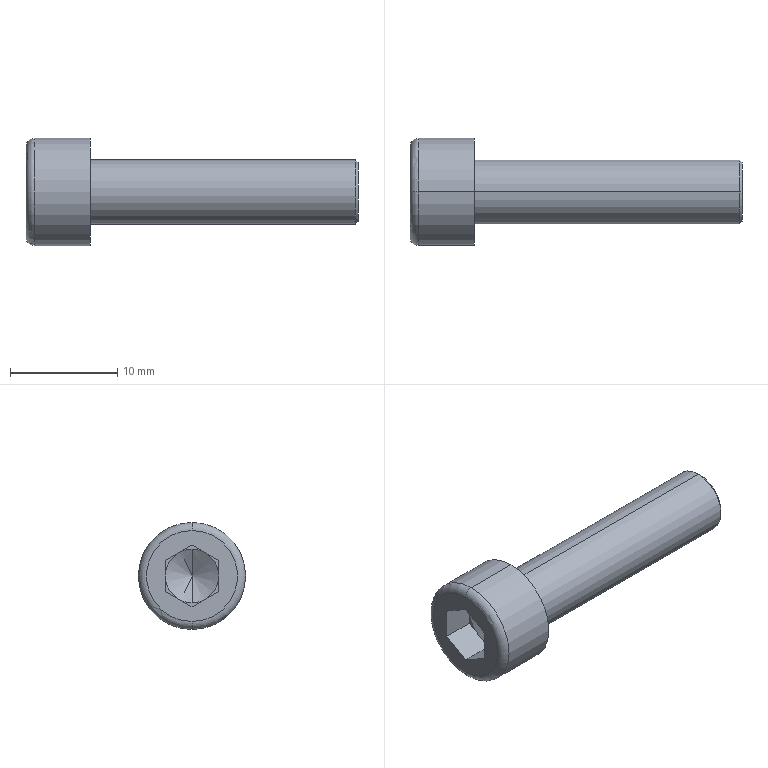Part | SolidWorks | features Fillet 2, RevCut 2, Boss 1, Chamfer 1, Cut 1, Extrusion 1, LPattern 1 | 1 solid | 25 faces | box 31 x 10 x 10 mm | volume 1099 mm3 | plane 15 | cone 4 | cylinder 4 | torus 2 | commonest cylinder face diameters 6 x2 10 x2
STEP:
#1=CARTESIAN_POINT('',(31.,0.,-2.75));
#2=VERTEX_POINT('',#1);
#3=CARTESIAN_POINT('',(31.,0.,2.75));
#4=VERTEX_POINT('',#3);
#5=CARTESIAN_POINT('',(31.,0.,0.));
#6=DIRECTION('',(1.,0.,0.));
#7=DIRECTION('',(0.,0.,-1.));
#8=AXIS2_PLACEMENT_3D('',#5,#6,#7);
#9=CIRCLE('',#8,2.75);
#10=EDGE_CURVE('',#2,#4,#9,.T.);
#11=ORIENTED_EDGE('',*,*,#10,.F.);
#12=CARTESIAN_POINT('',(30.75,0.,-3.));
#13=VERTEX_POINT('',#12);
#14=CARTESIAN_POINT('',(31.,0.,-2.75));
#15=DIRECTION('',(-0.7071,0.,-0.7071));
#16=VECTOR('',#15,1000.);
#17=LINE('',#14,#16);
#18=EDGE_CURVE('',#2,#13,#17,.T.);
#19=ORIENTED_EDGE('',*,*,#18,.T.);
#20=CARTESIAN_POINT('',(30.75,0.,3.));
#21=VERTEX_POINT('',#20);
#22=CARTESIAN_POINT('',(30.75,0.,0.));
#23=DIRECTION('',(-1.,0.,0.));
#24=DIRECTION('',(0.,0.,-1.));
#25=AXIS2_PLACEMENT_3D('',#22,#23,#24);
#26=CIRCLE('',#25,3.);
#27=EDGE_CURVE('',#21,#13,#26,.T.);
#28=ORIENTED_EDGE('',*,*,#27,.F.);
#29=CARTESIAN_POINT('',(31.,0.,2.75));
#30=DIRECTION('',(-0.7071,0.,0.7071));
#31=VECTOR('',#30,1000.);
#32=LINE('',#29,#31);
#33=EDGE_CURVE('',#4,#21,#32,.T.);
#34=ORIENTED_EDGE('',*,*,#33,.F.);
#35=EDGE_LOOP('',(#11,#19,#28,#34));
#36=FACE_OUTER_BOUND('',#35,.T.);
#37=CARTESIAN_POINT('',(31.,0.,0.));
#38=DIRECTION('',(-1.,0.,0.));
#39=DIRECTION('',(0.,0.,1.));
#40=AXIS2_PLACEMENT_3D('',#37,#38,#39);
#41=CONICAL_SURFACE('',#40,2.75,0.7854);
#42=ADVANCED_FACE('',(#36),#41,.T.);
#43=CARTESIAN_POINT('',(0.,0.,4.25));
#44=VERTEX_POINT('',#43);
#45=CARTESIAN_POINT('',(0.,0.,-4.25));
#46=VERTEX_POINT('',#45);
#47=CARTESIAN_POINT('',(0.,0.,0.));
#48=DIRECTION('',(-1.,0.,0.));
#49=DIRECTION('',(0.,0.,-1.));
#50=AXIS2_PLACEMENT_3D('',#47,#48,#49);
#51=CIRCLE('',#50,4.25);
#52=EDGE_CURVE('',#44,#46,#51,.T.);
#53=ORIENTED_EDGE('',*,*,#52,.F.);
#54=CARTESIAN_POINT('',(0.75,0.,5.));
#55=VERTEX_POINT('',#54);
#56=CARTESIAN_POINT('',(0.75,0.,4.25));
#57=DIRECTION('',(0.,1.,0.));
#58=DIRECTION('',(0.,0.,1.));
#59=AXIS2_PLACEMENT_3D('',#56,#57,#58);
#60=CIRCLE('',#59,0.75);
#61=EDGE_CURVE('',#44,#55,#60,.T.);
#62=ORIENTED_EDGE('',*,*,#61,.T.);
#63=CARTESIAN_POINT('',(0.75,0.,-5.));
#64=VERTEX_POINT('',#63);
#65=CARTESIAN_POINT('',(0.75,0.,0.));
#66=DIRECTION('',(1.,0.,0.));
#67=DIRECTION('',(0.,0.,-1.));
#68=AXIS2_PLACEMENT_3D('',#65,#66,#67);
#69=CIRCLE('',#68,5.);
#70=EDGE_CURVE('',#64,#55,#69,.T.);
#71=ORIENTED_EDGE('',*,*,#70,.F.);
#72=CARTESIAN_POINT('',(0.75,0.,-4.25));
#73=DIRECTION('',(0.,-1.,0.));
#74=DIRECTION('',(0.,0.,-1.));
#75=AXIS2_PLACEMENT_3D('',#72,#73,#74);
#76=CIRCLE('',#75,0.75);
#77=EDGE_CURVE('',#46,#64,#76,.T.);
#78=ORIENTED_EDGE('',*,*,#77,.F.);
#79=EDGE_LOOP('',(#53,#62,#71,#78));
#80=FACE_OUTER_BOUND('',#79,.T.);
#81=CARTESIAN_POINT('',(0.75,0.,0.));
#82=DIRECTION('',(1.,0.,0.));
#83=DIRECTION('',(0.,0.,-1.));
#84=AXIS2_PLACEMENT_3D('',#81,#82,#83);
#85=TOROIDAL_SURFACE('',#84,4.25,0.75);
#86=ADVANCED_FACE('',(#80),#85,.T.);
#87=CARTESIAN_POINT('',(4.443,0.,0.));
#88=VERTEX_POINT('',#87);
#89=CARTESIAN_POINT('',(3.,0.,2.5));
#90=VERTEX_POINT('',#89);
#91=CARTESIAN_POINT('',(3.,0.,2.5));
#92=DIRECTION('',(-0.5,0.,0.866));
#93=VECTOR('',#92,1000.);
#94=LINE('',#91,#93);
#95=EDGE_CURVE('',#88,#90,#94,.T.);
#96=ORIENTED_EDGE('',*,*,#95,.F.);
#97=CARTESIAN_POINT('',(3.,0.,-2.5));
#98=VERTEX_POINT('',#97);
#99=CARTESIAN_POINT('',(3.,0.,-2.5));
#100=DIRECTION('',(-0.5,0.,-0.866));
#101=VECTOR('',#100,1000.);
#102=LINE('',#99,#101);
#103=EDGE_CURVE('',#88,#98,#102,.T.);
#104=ORIENTED_EDGE('',*,*,#103,.T.);
#105=CARTESIAN_POINT('',(3.,-1.25,-2.165));
#106=VERTEX_POINT('',#105);
#107=CARTESIAN_POINT('',(3.,0.,0.));
#108=DIRECTION('',(1.,0.,0.));
#109=DIRECTION('',(0.,0.,1.));
#110=AXIS2_PLACEMENT_3D('',#107,#108,#109);
#111=CIRCLE('',#110,2.5);
#112=EDGE_CURVE('',#106,#98,#111,.T.);
#113=ORIENTED_EDGE('',*,*,#112,.F.);
#114=CARTESIAN_POINT('',(3.,-2.5,0.));
#115=VERTEX_POINT('',#114);
#116=CARTESIAN_POINT('',(3.,0.,0.));
#117=DIRECTION('',(1.,0.,0.));
#118=DIRECTION('',(0.,0.,1.));
#119=AXIS2_PLACEMENT_3D('',#116,#117,#118);
#120=CIRCLE('',#119,2.5);
#121=EDGE_CURVE('',#115,#106,#120,.T.);
#122=ORIENTED_EDGE('',*,*,#121,.F.);
#123=CARTESIAN_POINT('',(3.,-1.25,2.165));
#124=VERTEX_POINT('',#123);
#125=CARTESIAN_POINT('',(3.,0.,0.));
#126=DIRECTION('',(1.,0.,0.));
#127=DIRECTION('',(0.,0.,1.));
#128=AXIS2_PLACEMENT_3D('',#125,#126,#127);
#129=CIRCLE('',#128,2.5);
#130=EDGE_CURVE('',#124,#115,#129,.T.);
#131=ORIENTED_EDGE('',*,*,#130,.F.);
#132=CARTESIAN_POINT('',(3.,0.,0.));
#133=DIRECTION('',(1.,0.,0.));
#134=DIRECTION('',(0.,0.,1.));
#135=AXIS2_PLACEMENT_3D('',#132,#133,#134);
#136=CIRCLE('',#135,2.5);
#137=EDGE_CURVE('',#90,#124,#136,.T.);
#138=ORIENTED_EDGE('',*,*,#137,.F.);
#139=EDGE_LOOP('',(#96,#104,#113,#122,#131,#138));
#140=FACE_OUTER_BOUND('',#139,.T.);
#141=CARTESIAN_POINT('',(3.,0.,0.));
#142=DIRECTION('',(-1.,0.,0.));
#143=DIRECTION('',(0.,0.,1.));
#144=AXIS2_PLACEMENT_3D('',#141,#142,#143);
#145=CONICAL_SURFACE('',#144,2.5,1.047);
#146=ADVANCED_FACE('',(#140),#145,.F.);
#147=ORIENTED_EDGE('',*,*,#27,.T.);
#148=CARTESIAN_POINT('',(6.,0.,-3.));
#149=VERTEX_POINT('',#148);
#150=CARTESIAN_POINT('',(31.,0.,-3.));
#151=DIRECTION('',(-1.,0.,0.));
#152=VECTOR('',#151,1000.);
#153=LINE('',#150,#152);
#154=EDGE_CURVE('',#13,#149,#153,.T.);
#155=ORIENTED_EDGE('',*,*,#154,.T.);
#156=CARTESIAN_POINT('',(6.,0.,3.));
#157=VERTEX_POINT('',#156);
#158=CARTESIAN_POINT('',(6.,0.,0.));
#159=DIRECTION('',(1.,0.,0.));
#160=DIRECTION('',(0.,0.,-1.));
#161=AXIS2_PLACEMENT_3D('',#158,#159,#160);
#162=CIRCLE('',#161,3.);
#163=EDGE_CURVE('',#149,#157,#162,.T.);
#164=ORIENTED_EDGE('',*,*,#163,.T.);
#165=CARTESIAN_POINT('',(31.,0.,3.));
#166=DIRECTION('',(-1.,0.,0.));
#167=VECTOR('',#166,1000.);
#168=LINE('',#165,#167);
#169=EDGE_CURVE('',#21,#157,#168,.T.);
#170=ORIENTED_EDGE('',*,*,#169,.F.);
#171=EDGE_LOOP('',(#147,#155,#164,#170));
#172=FACE_OUTER_BOUND('',#171,.T.);
#173=CARTESIAN_POINT('',(31.,0.,0.));
#174=DIRECTION('',(-1.,0.,0.));
#175=DIRECTION('',(0.,0.,1.));
#176=AXIS2_PLACEMENT_3D('',#173,#174,#175);
#177=CYLINDRICAL_SURFACE('',#176,3.);
#178=ADVANCED_FACE('',(#172),#177,.T.);
#179=CARTESIAN_POINT('',(6.,0.,-5.));
#180=VERTEX_POINT('',#179);
#181=CARTESIAN_POINT('',(6.,0.,5.));
#182=VERTEX_POINT('',#181);
#183=CARTESIAN_POINT('',(6.,0.,0.));
#184=DIRECTION('',(1.,0.,0.));
#185=DIRECTION('',(0.,0.,-1.));
#186=AXIS2_PLACEMENT_3D('',#183,#184,#185);
#187=CIRCLE('',#186,5.);
#188=EDGE_CURVE('',#180,#182,#187,.T.);
#189=ORIENTED_EDGE('',*,*,#188,.F.);
#190=CARTESIAN_POINT('',(6.,0.,-5.));
#191=DIRECTION('',(-1.,0.,0.));
#192=VECTOR('',#191,1000.);
#193=LINE('',#190,#192);
#194=EDGE_CURVE('',#180,#64,#193,.T.);
#195=ORIENTED_EDGE('',*,*,#194,.T.);
#196=ORIENTED_EDGE('',*,*,#70,.T.);
#197=CARTESIAN_POINT('',(6.,0.,5.));
#198=DIRECTION('',(-1.,0.,0.));
#199=VECTOR('',#198,1000.);
#200=LINE('',#197,#199);
#201=EDGE_CURVE('',#182,#55,#200,.T.);
#202=ORIENTED_EDGE('',*,*,#201,.F.);
#203=EDGE_LOOP('',(#189,#195,#196,#202));
#204=FACE_OUTER_BOUND('',#203,.T.);
#205=CARTESIAN_POINT('',(6.,0.,0.));
#206=DIRECTION('',(-1.,0.,0.));
#207=DIRECTION('',(0.,0.,1.));
#208=AXIS2_PLACEMENT_3D('',#205,#206,#207);
#209=CYLINDRICAL_SURFACE('',#208,5.);
#210=ADVANCED_FACE('',(#204),#209,.T.);
#211=CARTESIAN_POINT('',(3.,-2.5,1.443));
#212=VERTEX_POINT('',#211);
#213=CARTESIAN_POINT('',(3.,0.,2.887));
#214=DIRECTION('',(0.,-0.866,-0.5));
#215=VECTOR('',#214,1000.);
#216=LINE('',#213,#215);
#217=EDGE_CURVE('',#124,#212,#216,.T.);
#218=ORIENTED_EDGE('',*,*,#217,.F.);
#219=ORIENTED_EDGE('',*,*,#130,.T.);
#220=CARTESIAN_POINT('',(3.,-2.5,1.443));
#221=DIRECTION('',(0.,0.,-1.));
#222=VECTOR('',#221,1000.);
#223=LINE('',#220,#222);
#224=EDGE_CURVE('',#212,#115,#223,.T.);
#225=ORIENTED_EDGE('',*,*,#224,.F.);
#226=EDGE_LOOP('',(#218,#219,#225));
#227=FACE_OUTER_BOUND('',#226,.T.);
#228=CARTESIAN_POINT('',(3.,-5.,0.));
#229=DIRECTION('',(-1.,0.,0.));
#230=DIRECTION('',(0.,0.,1.));
#231=AXIS2_PLACEMENT_3D('',#228,#229,#230);
#232=PLANE('',#231);
#233=ADVANCED_FACE('',(#227),#232,.T.);
#234=CARTESIAN_POINT('',(3.,-2.5,-1.443));
#235=VERTEX_POINT('',#234);
#236=CARTESIAN_POINT('',(3.,-2.5,1.443));
#237=DIRECTION('',(0.,0.,-1.));
#238=VECTOR('',#237,1000.);
#239=LINE('',#236,#238);
#240=EDGE_CURVE('',#115,#235,#239,.T.);
#241=ORIENTED_EDGE('',*,*,#240,.F.);
#242=ORIENTED_EDGE('',*,*,#121,.T.);
#243=CARTESIAN_POINT('',(3.,-2.5,-1.443));
#244=DIRECTION('',(0.,0.866,-0.5));
#245=VECTOR('',#244,1000.);
#246=LINE('',#243,#245);
#247=EDGE_CURVE('',#235,#106,#246,.T.);
#248=ORIENTED_EDGE('',*,*,#247,.F.);
#249=EDGE_LOOP('',(#241,#242,#248));
#250=FACE_OUTER_BOUND('',#249,.T.);
#251=CARTESIAN_POINT('',(3.,-5.,0.));
#252=DIRECTION('',(-1.,0.,0.));
#253=DIRECTION('',(0.,0.,1.));
#254=AXIS2_PLACEMENT_3D('',#251,#252,#253);
#255=PLANE('',#254);
#256=ADVANCED_FACE('',(#250),#255,.T.);
#257=CARTESIAN_POINT('',(3.,0.,-2.887));
#258=VERTEX_POINT('',#257);
#259=CARTESIAN_POINT('',(3.,-2.5,-1.443));
#260=DIRECTION('',(0.,0.866,-0.5));
#261=VECTOR('',#260,1000.);
#262=LINE('',#259,#261);
#263=EDGE_CURVE('',#106,#258,#262,.T.);
#264=ORIENTED_EDGE('',*,*,#263,.F.);
#265=ORIENTED_EDGE('',*,*,#112,.T.);
#266=CARTESIAN_POINT('',(3.,1.25,-2.165));
#267=VERTEX_POINT('',#266);
#268=CARTESIAN_POINT('',(3.,0.,0.));
#269=DIRECTION('',(1.,0.,0.));
#270=DIRECTION('',(0.,0.,1.));
#271=AXIS2_PLACEMENT_3D('',#268,#269,#270);
#272=CIRCLE('',#271,2.5);
#273=EDGE_CURVE('',#98,#267,#272,.T.);
#274=ORIENTED_EDGE('',*,*,#273,.T.);
#275=CARTESIAN_POINT('',(3.,0.,-2.887));
#276=DIRECTION('',(0.,0.866,0.5));
#277=VECTOR('',#276,1000.);
#278=LINE('',#275,#277);
#279=EDGE_CURVE('',#258,#267,#278,.T.);
#280=ORIENTED_EDGE('',*,*,#279,.F.);
#281=EDGE_LOOP('',(#264,#265,#274,#280));
#282=FACE_OUTER_BOUND('',#281,.T.);
#283=CARTESIAN_POINT('',(3.,-5.,0.));
#284=DIRECTION('',(-1.,0.,0.));
#285=DIRECTION('',(0.,0.,1.));
#286=AXIS2_PLACEMENT_3D('',#283,#284,#285);
#287=PLANE('',#286);
#288=ADVANCED_FACE('',(#282),#287,.T.);
#289=CARTESIAN_POINT('',(3.,2.5,-1.443));
#290=VERTEX_POINT('',#289);
#291=CARTESIAN_POINT('',(3.,0.,-2.887));
#292=DIRECTION('',(0.,0.866,0.5));
#293=VECTOR('',#292,1000.);
#294=LINE('',#291,#293);
#295=EDGE_CURVE('',#267,#290,#294,.T.);
#296=ORIENTED_EDGE('',*,*,#295,.F.);
#297=CARTESIAN_POINT('',(3.,2.5,0.));
#298=VERTEX_POINT('',#297);
#299=CARTESIAN_POINT('',(3.,0.,0.));
#300=DIRECTION('',(1.,0.,0.));
#301=DIRECTION('',(0.,0.,-1.));
#302=AXIS2_PLACEMENT_3D('',#299,#300,#301);
#303=CIRCLE('',#302,2.5);
#304=EDGE_CURVE('',#267,#298,#303,.T.);
#305=ORIENTED_EDGE('',*,*,#304,.T.);
#306=CARTESIAN_POINT('',(3.,2.5,-1.443));
#307=DIRECTION('',(0.,0.,1.));
#308=VECTOR('',#307,1000.);
#309=LINE('',#306,#308);
#310=EDGE_CURVE('',#290,#298,#309,.T.);
#311=ORIENTED_EDGE('',*,*,#310,.F.);
#312=EDGE_LOOP('',(#296,#305,#311));
#313=FACE_OUTER_BOUND('',#312,.T.);
#314=CARTESIAN_POINT('',(3.,-5.,0.));
#315=DIRECTION('',(-1.,0.,0.));
#316=DIRECTION('',(0.,0.,1.));
#317=AXIS2_PLACEMENT_3D('',#314,#315,#316);
#318=PLANE('',#317);
#319=ADVANCED_FACE('',(#313),#318,.T.);
#320=CARTESIAN_POINT('',(3.,2.5,1.443));
#321=VERTEX_POINT('',#320);
#322=CARTESIAN_POINT('',(3.,2.5,-1.443));
#323=DIRECTION('',(0.,0.,1.));
#324=VECTOR('',#323,1000.);
#325=LINE('',#322,#324);
#326=EDGE_CURVE('',#298,#321,#325,.T.);
#327=ORIENTED_EDGE('',*,*,#326,.F.);
#328=CARTESIAN_POINT('',(3.,1.25,2.165));
#329=VERTEX_POINT('',#328);
#330=CARTESIAN_POINT('',(3.,0.,0.));
#331=DIRECTION('',(1.,0.,0.));
#332=DIRECTION('',(0.,0.,1.));
#333=AXIS2_PLACEMENT_3D('',#330,#331,#332);
#334=CIRCLE('',#333,2.5);
#335=EDGE_CURVE('',#298,#329,#334,.T.);
#336=ORIENTED_EDGE('',*,*,#335,.T.);
#337=CARTESIAN_POINT('',(3.,2.5,1.443));
#338=DIRECTION('',(0.,-0.866,0.5));
#339=VECTOR('',#338,1000.);
#340=LINE('',#337,#339);
#341=EDGE_CURVE('',#321,#329,#340,.T.);
#342=ORIENTED_EDGE('',*,*,#341,.F.);
#343=EDGE_LOOP('',(#327,#336,#342));
#344=FACE_OUTER_BOUND('',#343,.T.);
#345=CARTESIAN_POINT('',(3.,-5.,0.));
#346=DIRECTION('',(-1.,0.,0.));
#347=DIRECTION('',(0.,0.,1.));
#348=AXIS2_PLACEMENT_3D('',#345,#346,#347);
#349=PLANE('',#348);
#350=ADVANCED_FACE('',(#344),#349,.T.);
#351=CARTESIAN_POINT('',(3.,0.,2.887));
#352=VERTEX_POINT('',#351);
#353=CARTESIAN_POINT('',(3.,2.5,1.443));
#354=DIRECTION('',(0.,-0.866,0.5));
#355=VECTOR('',#354,1000.);
#356=LINE('',#353,#355);
#357=EDGE_CURVE('',#329,#352,#356,.T.);
#358=ORIENTED_EDGE('',*,*,#357,.F.);
#359=CARTESIAN_POINT('',(3.,0.,0.));
#360=DIRECTION('',(1.,0.,0.));
#361=DIRECTION('',(0.,0.,1.));
#362=AXIS2_PLACEMENT_3D('',#359,#360,#361);
#363=CIRCLE('',#362,2.5);
#364=EDGE_CURVE('',#329,#90,#363,.T.);
#365=ORIENTED_EDGE('',*,*,#364,.T.);
#366=ORIENTED_EDGE('',*,*,#137,.T.);
#367=CARTESIAN_POINT('',(3.,0.,2.887));
#368=DIRECTION('',(0.,-0.866,-0.5));
#369=VECTOR('',#368,1000.);
#370=LINE('',#367,#369);
#371=EDGE_CURVE('',#352,#124,#370,.T.);
#372=ORIENTED_EDGE('',*,*,#371,.F.);
#373=EDGE_LOOP('',(#358,#365,#366,#372));
#374=FACE_OUTER_BOUND('',#373,.T.);
#375=CARTESIAN_POINT('',(3.,-5.,0.));
#376=DIRECTION('',(-1.,0.,0.));
#377=DIRECTION('',(0.,0.,1.));
#378=AXIS2_PLACEMENT_3D('',#375,#376,#377);
#379=PLANE('',#378);
#380=ADVANCED_FACE('',(#374),#379,.T.);
#381=CARTESIAN_POINT('',(0.,0.,0.));
#382=DIRECTION('',(-1.,0.,0.));
#383=DIRECTION('',(0.,0.,-1.));
#384=AXIS2_PLACEMENT_3D('',#381,#382,#383);
#385=CIRCLE('',#384,4.25);
#386=EDGE_CURVE('',#46,#44,#385,.T.);
#387=ORIENTED_EDGE('',*,*,#386,.T.);
#388=ORIENTED_EDGE('',*,*,#52,.T.);
#389=EDGE_LOOP('',(#387,#388));
#390=FACE_OUTER_BOUND('',#389,.T.);
#391=CARTESIAN_POINT('',(0.,-2.5,-1.443));
#392=VERTEX_POINT('',#391);
#393=CARTESIAN_POINT('',(0.,0.,-2.887));
#394=VERTEX_POINT('',#393);
#395=CARTESIAN_POINT('',(0.,-2.5,-1.443));
#396=DIRECTION('',(0.,0.866,-0.5));
#397=VECTOR('',#396,1000.);
#398=LINE('',#395,#397);
#399=EDGE_CURVE('',#392,#394,#398,.T.);
#400=ORIENTED_EDGE('',*,*,#399,.T.);
#401=CARTESIAN_POINT('',(0.,2.5,-1.443));
#402=VERTEX_POINT('',#401);
#403=CARTESIAN_POINT('',(0.,0.,-2.887));
#404=DIRECTION('',(0.,0.866,0.5));
#405=VECTOR('',#404,1000.);
#406=LINE('',#403,#405);
#407=EDGE_CURVE('',#394,#402,#406,.T.);
#408=ORIENTED_EDGE('',*,*,#407,.T.);
#409=CARTESIAN_POINT('',(0.,2.5,1.443));
#410=VERTEX_POINT('',#409);
#411=CARTESIAN_POINT('',(0.,2.5,-1.443));
#412=DIRECTION('',(0.,0.,1.));
#413=VECTOR('',#412,1000.);
#414=LINE('',#411,#413);
#415=EDGE_CURVE('',#402,#410,#414,.T.);
#416=ORIENTED_EDGE('',*,*,#415,.T.);
#417=CARTESIAN_POINT('',(0.,0.,2.887));
#418=VERTEX_POINT('',#417);
#419=CARTESIAN_POINT('',(0.,2.5,1.443));
#420=DIRECTION('',(0.,-0.866,0.5));
#421=VECTOR('',#420,1000.);
#422=LINE('',#419,#421);
#423=EDGE_CURVE('',#410,#418,#422,.T.);
#424=ORIENTED_EDGE('',*,*,#423,.T.);
#425=CARTESIAN_POINT('',(0.,-2.5,1.443));
#426=VERTEX_POINT('',#425);
#427=CARTESIAN_POINT('',(0.,0.,2.887));
#428=DIRECTION('',(0.,-0.866,-0.5));
#429=VECTOR('',#428,1000.);
#430=LINE('',#427,#429);
#431=EDGE_CURVE('',#418,#426,#430,.T.);
#432=ORIENTED_EDGE('',*,*,#431,.T.);
#433=CARTESIAN_POINT('',(0.,-2.5,1.443));
#434=DIRECTION('',(0.,0.,-1.));
#435=VECTOR('',#434,1000.);
#436=LINE('',#433,#435);
#437=EDGE_CURVE('',#426,#392,#436,.T.);
#438=ORIENTED_EDGE('',*,*,#437,.T.);
#439=EDGE_LOOP('',(#400,#408,#416,#424,#432,#438));
#440=FACE_BOUND('',#439,.T.);
#441=CARTESIAN_POINT('',(0.,0.,0.));
#442=DIRECTION('',(1.,0.,0.));
#443=DIRECTION('',(0.,0.,-1.));
#444=AXIS2_PLACEMENT_3D('',#441,#442,#443);
#445=PLANE('',#444);
#446=ADVANCED_FACE('',(#390,#440),#445,.F.);
#447=CARTESIAN_POINT('',(6.,0.,0.));
#448=DIRECTION('',(1.,0.,0.));
#449=DIRECTION('',(0.,0.,-1.));
#450=AXIS2_PLACEMENT_3D('',#447,#448,#449);
#451=CIRCLE('',#450,5.);
#452=EDGE_CURVE('',#182,#180,#451,.T.);
#453=ORIENTED_EDGE('',*,*,#452,.T.);
#454=ORIENTED_EDGE('',*,*,#188,.T.);
#455=EDGE_LOOP('',(#453,#454));
#456=FACE_OUTER_BOUND('',#455,.T.);
#457=CARTESIAN_POINT('',(6.,0.,0.));
#458=DIRECTION('',(1.,0.,0.));
#459=DIRECTION('',(0.,0.,-1.));
#460=AXIS2_PLACEMENT_3D('',#457,#458,#459);
#461=CIRCLE('',#460,3.);
#462=EDGE_CURVE('',#157,#149,#461,.T.);
#463=ORIENTED_EDGE('',*,*,#462,.F.);
#464=ORIENTED_EDGE('',*,*,#163,.F.);
#465=EDGE_LOOP('',(#463,#464));
#466=FACE_BOUND('',#465,.T.);
#467=CARTESIAN_POINT('',(6.,0.,0.));
#468=DIRECTION('',(1.,0.,0.));
#469=DIRECTION('',(0.,0.,-1.));
#470=AXIS2_PLACEMENT_3D('',#467,#468,#469);
#471=PLANE('',#470);
#472=ADVANCED_FACE('',(#456,#466),#471,.T.);
#473=ORIENTED_EDGE('',*,*,#194,.F.);
#474=ORIENTED_EDGE('',*,*,#452,.F.);
#475=ORIENTED_EDGE('',*,*,#201,.T.);
#476=CARTESIAN_POINT('',(0.75,0.,0.));
#477=DIRECTION('',(1.,0.,0.));
#478=DIRECTION('',(0.,0.,-1.));
#479=AXIS2_PLACEMENT_3D('',#476,#477,#478);
#480=CIRCLE('',#479,5.);
#481=EDGE_CURVE('',#55,#64,#480,.T.);
#482=ORIENTED_EDGE('',*,*,#481,.T.);
#483=EDGE_LOOP('',(#473,#474,#475,#482));
#484=FACE_OUTER_BOUND('',#483,.T.);
#485=CARTESIAN_POINT('',(6.,0.,0.));
#486=DIRECTION('',(-1.,0.,0.));
#487=DIRECTION('',(0.,0.,1.));
#488=AXIS2_PLACEMENT_3D('',#485,#486,#487);
#489=CYLINDRICAL_SURFACE('',#488,5.);
#490=ADVANCED_FACE('',(#484),#489,.T.);
#491=ORIENTED_EDGE('',*,*,#154,.F.);
#492=CARTESIAN_POINT('',(30.75,0.,0.));
#493=DIRECTION('',(-1.,0.,0.));
#494=DIRECTION('',(0.,0.,-1.));
#495=AXIS2_PLACEMENT_3D('',#492,#493,#494);
#496=CIRCLE('',#495,3.);
#497=EDGE_CURVE('',#13,#21,#496,.T.);
#498=ORIENTED_EDGE('',*,*,#497,.T.);
#499=ORIENTED_EDGE('',*,*,#169,.T.);
#500=ORIENTED_EDGE('',*,*,#462,.T.);
#501=EDGE_LOOP('',(#491,#498,#499,#500));
#502=FACE_OUTER_BOUND('',#501,.T.);
#503=CARTESIAN_POINT('',(31.,0.,0.));
#504=DIRECTION('',(-1.,0.,0.));
#505=DIRECTION('',(0.,0.,1.));
#506=AXIS2_PLACEMENT_3D('',#503,#504,#505);
#507=CYLINDRICAL_SURFACE('',#506,3.);
#508=ADVANCED_FACE('',(#502),#507,.T.);
#509=CARTESIAN_POINT('',(31.,0.,0.));
#510=DIRECTION('',(1.,0.,0.));
#511=DIRECTION('',(0.,0.,-1.));
#512=AXIS2_PLACEMENT_3D('',#509,#510,#511);
#513=CIRCLE('',#512,2.75);
#514=EDGE_CURVE('',#4,#2,#513,.T.);
#515=ORIENTED_EDGE('',*,*,#514,.T.);
#516=ORIENTED_EDGE('',*,*,#10,.T.);
#517=EDGE_LOOP('',(#515,#516));
#518=FACE_OUTER_BOUND('',#517,.T.);
#519=CARTESIAN_POINT('',(31.,0.,0.));
#520=DIRECTION('',(1.,0.,0.));
#521=DIRECTION('',(0.,0.,-1.));
#522=AXIS2_PLACEMENT_3D('',#519,#520,#521);
#523=PLANE('',#522);
#524=ADVANCED_FACE('',(#518),#523,.T.);
#525=ORIENTED_EDGE('',*,*,#399,.F.);
#526=CARTESIAN_POINT('',(3.,-2.5,-1.443));
#527=DIRECTION('',(-1.,0.,0.));
#528=VECTOR('',#527,1000.);
#529=LINE('',#526,#528);
#530=EDGE_CURVE('',#235,#392,#529,.T.);
#531=ORIENTED_EDGE('',*,*,#530,.F.);
#532=ORIENTED_EDGE('',*,*,#247,.T.);
#533=ORIENTED_EDGE('',*,*,#263,.T.);
#534=CARTESIAN_POINT('',(3.,0.,-2.887));
#535=DIRECTION('',(-1.,0.,0.));
#536=VECTOR('',#535,1000.);
#537=LINE('',#534,#536);
#538=EDGE_CURVE('',#258,#394,#537,.T.);
#539=ORIENTED_EDGE('',*,*,#538,.T.);
#540=EDGE_LOOP('',(#525,#531,#532,#533,#539));
#541=FACE_OUTER_BOUND('',#540,.T.);
#542=CARTESIAN_POINT('',(3.,-2.5,-1.443));
#543=DIRECTION('',(0.,0.5,0.866));
#544=DIRECTION('',(0.,-0.866,0.5));
#545=AXIS2_PLACEMENT_3D('',#542,#543,#544);
#546=PLANE('',#545);
#547=ADVANCED_FACE('',(#541),#546,.T.);
#548=ORIENTED_EDGE('',*,*,#407,.F.);
#549=ORIENTED_EDGE('',*,*,#538,.F.);
#550=ORIENTED_EDGE('',*,*,#279,.T.);
#551=ORIENTED_EDGE('',*,*,#295,.T.);
#552=CARTESIAN_POINT('',(3.,2.5,-1.443));
#553=DIRECTION('',(-1.,0.,0.));
#554=VECTOR('',#553,1000.);
#555=LINE('',#552,#554);
#556=EDGE_CURVE('',#290,#402,#555,.T.);
#557=ORIENTED_EDGE('',*,*,#556,.T.);
#558=EDGE_LOOP('',(#548,#549,#550,#551,#557));
#559=FACE_OUTER_BOUND('',#558,.T.);
#560=CARTESIAN_POINT('',(3.,0.,-2.887));
#561=DIRECTION('',(0.,-0.5,0.866));
#562=DIRECTION('',(0.,-0.866,-0.5));
#563=AXIS2_PLACEMENT_3D('',#560,#561,#562);
#564=PLANE('',#563);
#565=ADVANCED_FACE('',(#559),#564,.T.);
#566=ORIENTED_EDGE('',*,*,#415,.F.);
#567=ORIENTED_EDGE('',*,*,#556,.F.);
#568=ORIENTED_EDGE('',*,*,#310,.T.);
#569=ORIENTED_EDGE('',*,*,#326,.T.);
#570=CARTESIAN_POINT('',(3.,2.5,1.443));
#571=DIRECTION('',(-1.,0.,0.));
#572=VECTOR('',#571,1000.);
#573=LINE('',#570,#572);
#574=EDGE_CURVE('',#321,#410,#573,.T.);
#575=ORIENTED_EDGE('',*,*,#574,.T.);
#576=EDGE_LOOP('',(#566,#567,#568,#569,#575));
#577=FACE_OUTER_BOUND('',#576,.T.);
#578=CARTESIAN_POINT('',(3.,2.5,-1.443));
#579=DIRECTION('',(0.,-1.,0.));
#580=DIRECTION('',(0.,0.,-1.));
#581=AXIS2_PLACEMENT_3D('',#578,#579,#580);
#582=PLANE('',#581);
#583=ADVANCED_FACE('',(#577),#582,.T.);
#584=ORIENTED_EDGE('',*,*,#423,.F.);
#585=ORIENTED_EDGE('',*,*,#574,.F.);
#586=ORIENTED_EDGE('',*,*,#341,.T.);
#587=ORIENTED_EDGE('',*,*,#357,.T.);
#588=CARTESIAN_POINT('',(3.,0.,2.887));
#589=DIRECTION('',(-1.,0.,0.));
#590=VECTOR('',#589,1000.);
#591=LINE('',#588,#590);
#592=EDGE_CURVE('',#352,#418,#591,.T.);
#593=ORIENTED_EDGE('',*,*,#592,.T.);
#594=EDGE_LOOP('',(#584,#585,#586,#587,#593));
#595=FACE_OUTER_BOUND('',#594,.T.);
#596=CARTESIAN_POINT('',(3.,2.5,1.443));
#597=DIRECTION('',(0.,-0.5,-0.866));
#598=DIRECTION('',(0.,0.866,-0.5));
#599=AXIS2_PLACEMENT_3D('',#596,#597,#598);
#600=PLANE('',#599);
#601=ADVANCED_FACE('',(#595),#600,.T.);
#602=ORIENTED_EDGE('',*,*,#431,.F.);
#603=ORIENTED_EDGE('',*,*,#592,.F.);
#604=ORIENTED_EDGE('',*,*,#371,.T.);
#605=ORIENTED_EDGE('',*,*,#217,.T.);
#606=CARTESIAN_POINT('',(3.,-2.5,1.443));
#607=DIRECTION('',(-1.,0.,0.));
#608=VECTOR('',#607,1000.);
#609=LINE('',#606,#608);
#610=EDGE_CURVE('',#212,#426,#609,.T.);
#611=ORIENTED_EDGE('',*,*,#610,.T.);
#612=EDGE_LOOP('',(#602,#603,#604,#605,#611));
#613=FACE_OUTER_BOUND('',#612,.T.);
#614=CARTESIAN_POINT('',(3.,0.,2.887));
#615=DIRECTION('',(0.,0.5,-0.866));
#616=DIRECTION('',(0.,0.866,0.5));
#617=AXIS2_PLACEMENT_3D('',#614,#615,#616);
#618=PLANE('',#617);
#619=ADVANCED_FACE('',(#613),#618,.T.);
#620=ORIENTED_EDGE('',*,*,#437,.F.);
#621=ORIENTED_EDGE('',*,*,#610,.F.);
#622=ORIENTED_EDGE('',*,*,#224,.T.);
#623=ORIENTED_EDGE('',*,*,#240,.T.);
#624=ORIENTED_EDGE('',*,*,#530,.T.);
#625=EDGE_LOOP('',(#620,#621,#622,#623,#624));
#626=FACE_OUTER_BOUND('',#625,.T.);
#627=CARTESIAN_POINT('',(3.,-2.5,1.443));
#628=DIRECTION('',(0.,1.,0.));
#629=DIRECTION('',(0.,0.,1.));
#630=AXIS2_PLACEMENT_3D('',#627,#628,#629);
#631=PLANE('',#630);
#632=ADVANCED_FACE('',(#626),#631,.T.);
#633=ORIENTED_EDGE('',*,*,#103,.F.);
#634=ORIENTED_EDGE('',*,*,#95,.T.);
#635=ORIENTED_EDGE('',*,*,#364,.F.);
#636=ORIENTED_EDGE('',*,*,#335,.F.);
#637=ORIENTED_EDGE('',*,*,#304,.F.);
#638=ORIENTED_EDGE('',*,*,#273,.F.);
#639=EDGE_LOOP('',(#633,#634,#635,#636,#637,#638));
#640=FACE_OUTER_BOUND('',#639,.T.);
#641=CARTESIAN_POINT('',(3.,0.,0.));
#642=DIRECTION('',(-1.,0.,0.));
#643=DIRECTION('',(0.,0.,1.));
#644=AXIS2_PLACEMENT_3D('',#641,#642,#643);
#645=CONICAL_SURFACE('',#644,2.5,1.047);
#646=ADVANCED_FACE('',(#640),#645,.F.);
#647=ORIENTED_EDGE('',*,*,#61,.F.);
#648=ORIENTED_EDGE('',*,*,#386,.F.);
#649=ORIENTED_EDGE('',*,*,#77,.T.);
#650=ORIENTED_EDGE('',*,*,#481,.F.);
#651=EDGE_LOOP('',(#647,#648,#649,#650));
#652=FACE_OUTER_BOUND('',#651,.T.);
#653=CARTESIAN_POINT('',(0.75,0.,0.));
#654=DIRECTION('',(1.,0.,0.));
#655=DIRECTION('',(0.,0.,-1.));
#656=AXIS2_PLACEMENT_3D('',#653,#654,#655);
#657=TOROIDAL_SURFACE('',#656,4.25,0.75);
#658=ADVANCED_FACE('',(#652),#657,.T.);
#659=ORIENTED_EDGE('',*,*,#18,.F.);
#660=ORIENTED_EDGE('',*,*,#514,.F.);
#661=ORIENTED_EDGE('',*,*,#33,.T.);
#662=ORIENTED_EDGE('',*,*,#497,.F.);
#663=EDGE_LOOP('',(#659,#660,#661,#662));
#664=FACE_OUTER_BOUND('',#663,.T.);
#665=CARTESIAN_POINT('',(31.,0.,0.));
#666=DIRECTION('',(-1.,0.,0.));
#667=DIRECTION('',(0.,0.,1.));
#668=AXIS2_PLACEMENT_3D('',#665,#666,#667);
#669=CONICAL_SURFACE('',#668,2.75,0.7854);
#670=ADVANCED_FACE('',(#664),#669,.T.);
#671=CLOSED_SHELL('',(#42,#86,#146,#178,#210,#233,#256,#288,#319,#350,#380,#446,#472,#490,#508,#524,#547,#565,#583,#601,#619,#632,#646,#658,#670));
#672=MANIFOLD_SOLID_BREP('',#671);
#673=CARTESIAN_POINT('',(0.,0.,0.));
#674=DIRECTION('',(0.,0.,1.));
#675=DIRECTION('',(1.,0.,0.));
#676=AXIS2_PLACEMENT_3D('',#673,#674,#675);
#677=(LENGTH_UNIT()NAMED_UNIT(*)SI_UNIT(.MILLI.,.METRE.));
#678=UNCERTAINTY_MEASURE_WITH_UNIT(LENGTH_MEASURE(0.00001),#677,'','');
#679=(NAMED_UNIT(*)PLANE_ANGLE_UNIT()SI_UNIT($,.RADIAN.));
#680=(NAMED_UNIT(*)SI_UNIT($,.STERADIAN.)SOLID_ANGLE_UNIT());
#681=(GEOMETRIC_REPRESENTATION_CONTEXT(3)GLOBAL_UNCERTAINTY_ASSIGNED_CONTEXT((#678))GLOBAL_UNIT_ASSIGNED_CONTEXT((#677,#679,#680))REPRESENTATION_CONTEXT('',''));
#682=ADVANCED_BREP_SHAPE_REPRESENTATION('',(#672,#676),#681);